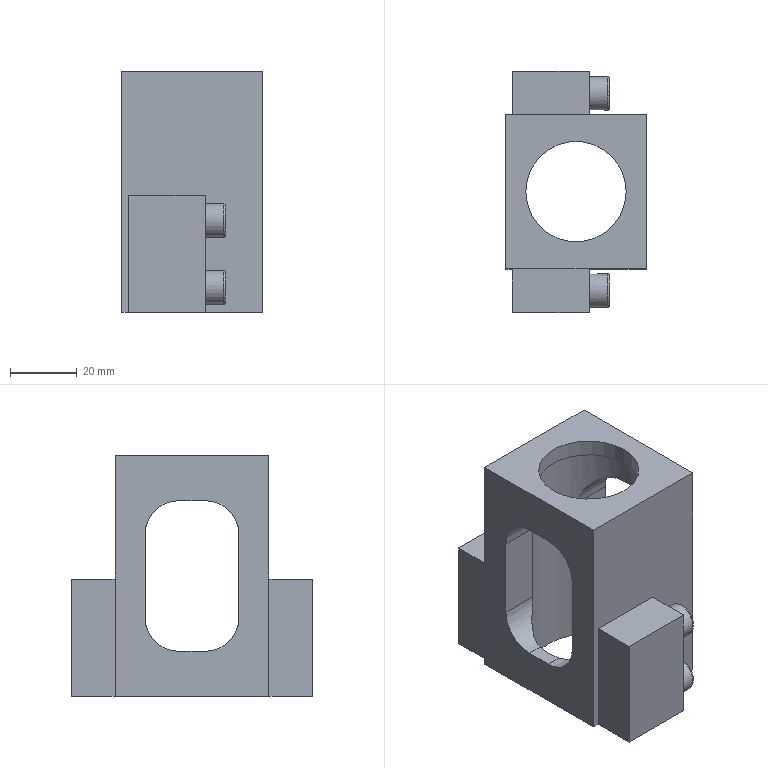Part | NX | features BREP 8, DATUM_CSYS 6, SKETCH 5, EXTRUDE 4, META 4, Container 1, EXTRACT_BODY 1, Geometry Instance 1, UNITE 1 | 5 solids | 121 faces | box 42 x 72 x 72 mm | volume 82827 mm3 | plane 79 | cylinder 30 | cone 8 | torus 4 | commonest cylinder face diameters 6 x8 20 x8 5 x4 5.7 x4 10 x4 30 x1